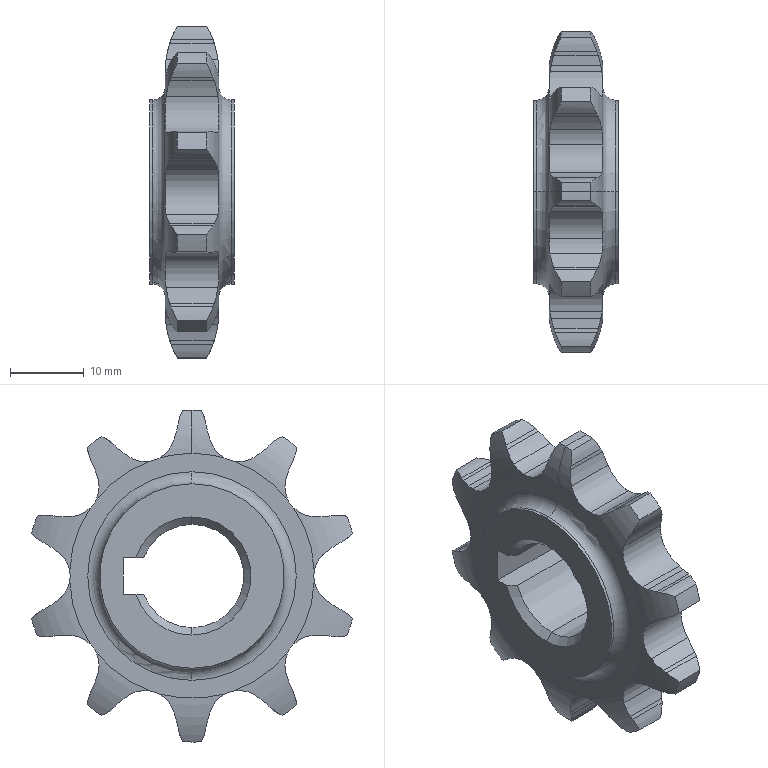Part | SolidWorks | features BaseBody 1 | 1 solid | 133 faces | box 11.39 x 43.493 x 45 mm | volume 8237 mm3 | cylinder 74 | plane 27 | torus 26 | cone 6 | commonest cylinder face diameters 11.885 x22 20.732 x22 8.06 x12 45 x11 25 x4 14 x3